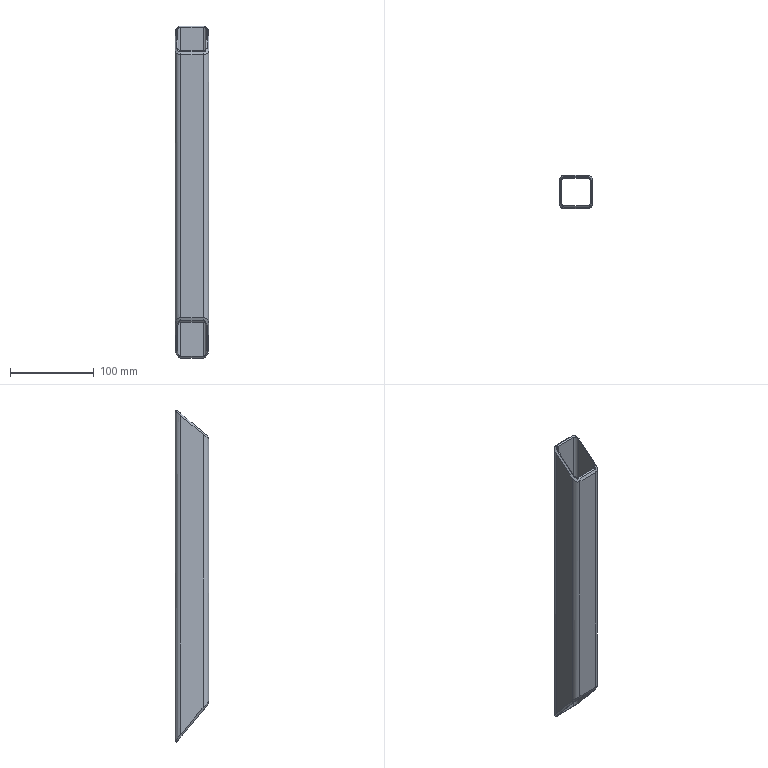Part | STEP file | 1 | 1 solid | 42 faces | box 40 x 40 x 397.182 mm | volume 149500 mm3 | plane 18 | spline 16 | cylinder 8 | commonest cylinder face diameters 7.2 x4 13.2 x4